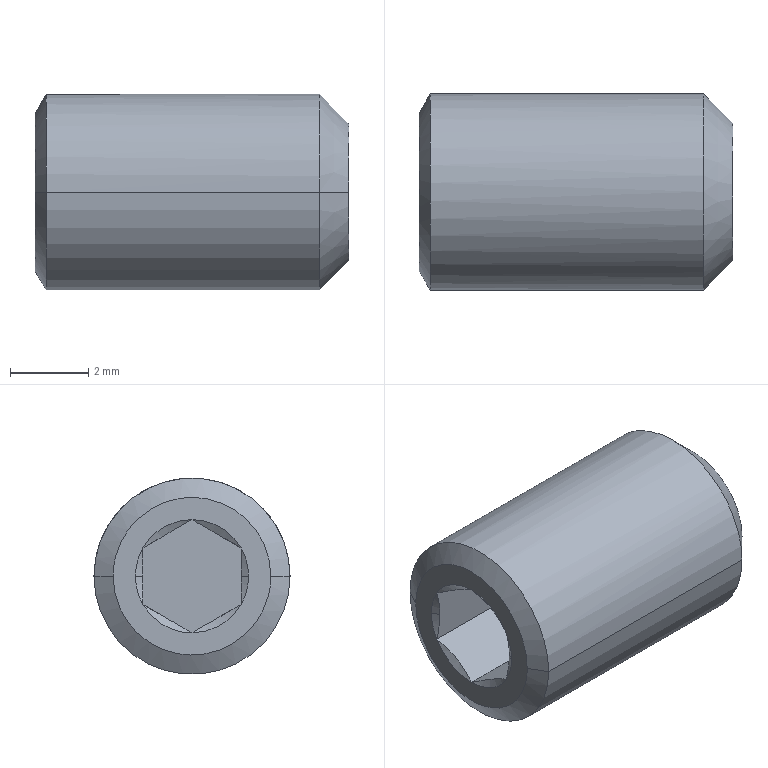Part | STEP file | _Headless pin DIN 913 - M5x8 | 1 solid | 23 faces | box 8 x 5 x 5 mm | volume 135.796 mm3 | cone 12 | plane 9 | cylinder 2 | commonest cylinder face diameters 5 x2